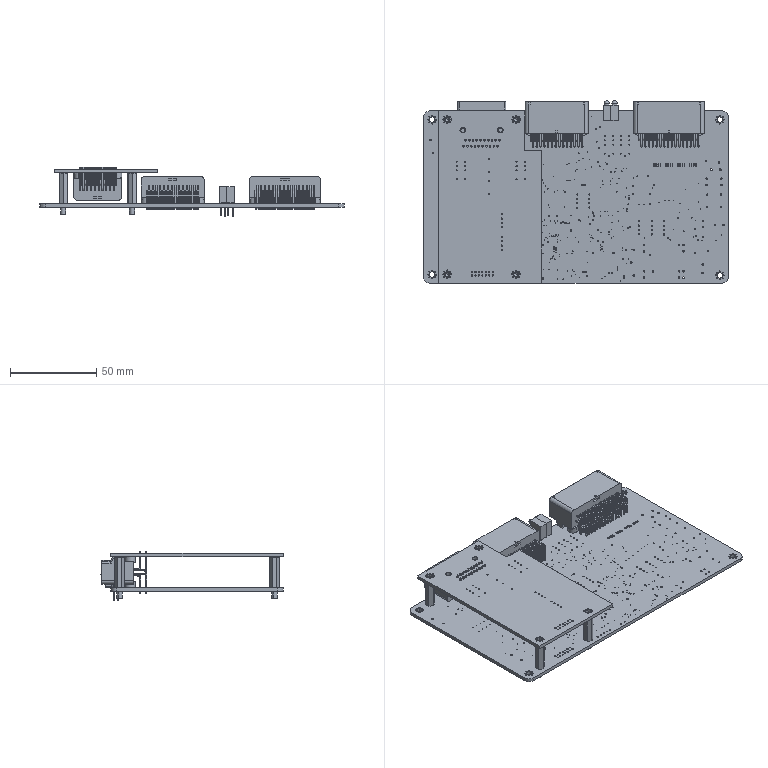Part | SolidWorks | 11 solids | 3514 faces | volume 62246 mm3 | plane 1794 | cylinder 1694 | cone 24 | sphere 2 | commonest cylinder face diameters 0.305 x670 0.6 x192 0.381 x136 0.7 x120 1 x110 0.889 x104